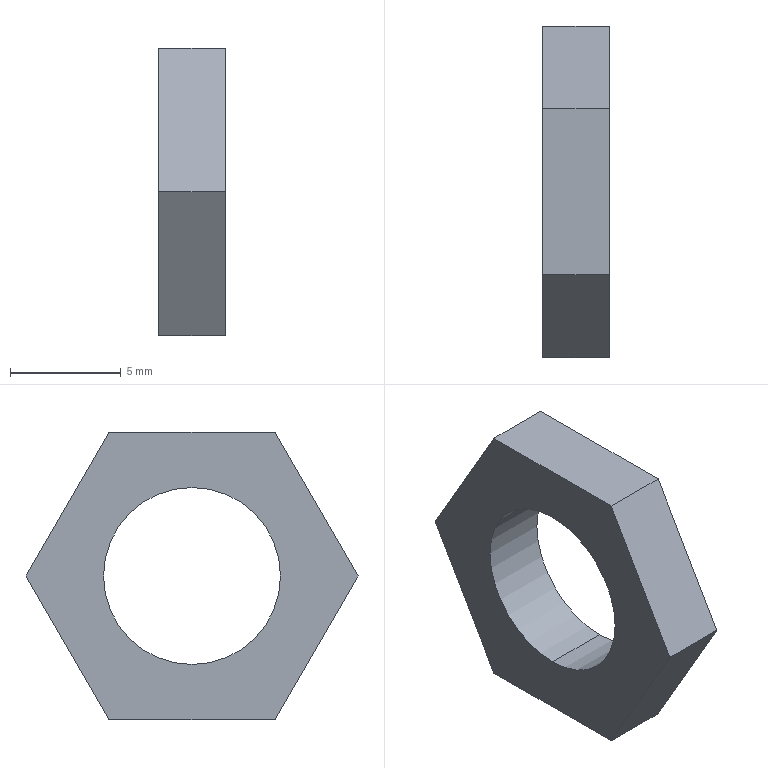Part | STEP file | E2E_X2D1_N_NUT | 1 solid | 10 faces | box 3 x 15.011 x 13 mm | volume 288.278 mm3 | plane 8 | cylinder 2 | commonest cylinder face diameters 8 x2
STEP:
#1=CARTESIAN_POINT('',(0.,0.,0.));
#2=DIRECTION('',(0.,0.,1.));
#3=DIRECTION('',(1.,0.,0.));
#4=AXIS2_PLACEMENT_3D('',#1,#2,#3);
#5=CARTESIAN_POINT('',(3.,0.,4.));
#6=VERTEX_POINT('',#5);
#7=CARTESIAN_POINT('',(0.,0.,4.));
#8=VERTEX_POINT('',#7);
#9=CARTESIAN_POINT('',(3.,0.,4.));
#10=DIRECTION('',(-1.,0.,0.));
#11=VECTOR('',#10,1.);
#12=LINE('',#9,#11);
#13=CARTESIAN_POINT('',(3.,0.,0.));
#14=DIRECTION('',(-1.,0.,0.));
#15=DIRECTION('',(0.,0.,1.));
#16=AXIS2_PLACEMENT_3D('',#13,#14,#15);
#17=CYLINDRICAL_SURFACE('',#16,4.);
#18=CARTESIAN_POINT('',(6.283,0.));
#19=DIRECTION('',(0.,1.));
#20=VECTOR('',#19,1.);
#21=LINE('',#18,#20);
#22=(GEOMETRIC_REPRESENTATION_CONTEXT(2)PARAMETRIC_REPRESENTATION_CONTEXT()REPRESENTATION_CONTEXT('',''));
#23=DEFINITIONAL_REPRESENTATION('',(#21),#22);
#24=PCURVE('',#17,#23);
#25=CARTESIAN_POINT('',(3.,0.,0.));
#26=DIRECTION('',(-1.,0.,0.));
#27=DIRECTION('',(0.,0.,1.));
#28=AXIS2_PLACEMENT_3D('',#25,#26,#27);
#29=CYLINDRICAL_SURFACE('',#28,4.);
#30=CARTESIAN_POINT('',(0.,0.));
#31=DIRECTION('',(0.,1.));
#32=VECTOR('',#31,1.);
#33=LINE('',#30,#32);
#34=(GEOMETRIC_REPRESENTATION_CONTEXT(2)PARAMETRIC_REPRESENTATION_CONTEXT()REPRESENTATION_CONTEXT('',''));
#35=DEFINITIONAL_REPRESENTATION('',(#33),#34);
#36=PCURVE('',#29,#35);
#37=SURFACE_CURVE('',#12,(#24,#36),.PCURVE_S1.);
#38=EDGE_CURVE('',#6,#8,#37,.T.);
#39=ORIENTED_EDGE('',*,*,#38,.T.);
#40=CARTESIAN_POINT('',(0.,0.,-4.));
#41=VERTEX_POINT('',#40);
#42=CARTESIAN_POINT('',(0.,0.,0.));
#43=DIRECTION('',(1.,0.,0.));
#44=DIRECTION('',(0.,0.,-1.));
#45=AXIS2_PLACEMENT_3D('',#42,#43,#44);
#46=CIRCLE('',#45,4.);
#47=CARTESIAN_POINT('',(9.425,3.));
#48=DIRECTION('',(-1.,0.));
#49=VECTOR('',#48,1.);
#50=LINE('',#47,#49);
#51=(GEOMETRIC_REPRESENTATION_CONTEXT(2)PARAMETRIC_REPRESENTATION_CONTEXT()REPRESENTATION_CONTEXT('',''));
#52=DEFINITIONAL_REPRESENTATION('',(#50),#51);
#53=PCURVE('',#17,#52);
#54=CARTESIAN_POINT('',(0.,-3.753,-6.5));
#55=DIRECTION('',(1.,0.,0.));
#56=DIRECTION('',(0.,0.,-1.));
#57=AXIS2_PLACEMENT_3D('',#54,#55,#56);
#58=PLANE('',#57);
#59=CARTESIAN_POINT('',(-6.5,3.753));
#60=DIRECTION('',(1.,0.));
#61=AXIS2_PLACEMENT_2D('',#59,#60);
#62=CIRCLE('',#61,4.);
#63=(GEOMETRIC_REPRESENTATION_CONTEXT(2)PARAMETRIC_REPRESENTATION_CONTEXT()REPRESENTATION_CONTEXT('',''));
#64=DEFINITIONAL_REPRESENTATION('',(#62),#63);
#65=PCURVE('',#58,#64);
#66=SURFACE_CURVE('',#46,(#53,#65),.PCURVE_S1.);
#67=EDGE_CURVE('',#8,#41,#66,.T.);
#68=ORIENTED_EDGE('',*,*,#67,.T.);
#69=CARTESIAN_POINT('',(3.,0.,-4.));
#70=VERTEX_POINT('',#69);
#71=CARTESIAN_POINT('',(3.,0.,-4.));
#72=DIRECTION('',(-1.,0.,0.));
#73=VECTOR('',#72,1.);
#74=LINE('',#71,#73);
#75=CARTESIAN_POINT('',(3.142,0.));
#76=DIRECTION('',(0.,1.));
#77=VECTOR('',#76,1.);
#78=LINE('',#75,#77);
#79=(GEOMETRIC_REPRESENTATION_CONTEXT(2)PARAMETRIC_REPRESENTATION_CONTEXT()REPRESENTATION_CONTEXT('',''));
#80=DEFINITIONAL_REPRESENTATION('',(#78),#79);
#81=PCURVE('',#17,#80);
#82=CARTESIAN_POINT('',(3.142,0.));
#83=DIRECTION('',(0.,1.));
#84=VECTOR('',#83,1.);
#85=LINE('',#82,#84);
#86=(GEOMETRIC_REPRESENTATION_CONTEXT(2)PARAMETRIC_REPRESENTATION_CONTEXT()REPRESENTATION_CONTEXT('',''));
#87=DEFINITIONAL_REPRESENTATION('',(#85),#86);
#88=PCURVE('',#29,#87);
#89=SURFACE_CURVE('',#74,(#81,#88),.PCURVE_S1.);
#90=EDGE_CURVE('',#70,#41,#89,.T.);
#91=ORIENTED_EDGE('',*,*,#90,.F.);
#92=CARTESIAN_POINT('',(3.,0.,0.));
#93=DIRECTION('',(1.,0.,0.));
#94=DIRECTION('',(0.,0.,-1.));
#95=AXIS2_PLACEMENT_3D('',#92,#93,#94);
#96=CIRCLE('',#95,4.);
#97=CARTESIAN_POINT('',(9.425,0.));
#98=DIRECTION('',(-1.,0.));
#99=VECTOR('',#98,1.);
#100=LINE('',#97,#99);
#101=(GEOMETRIC_REPRESENTATION_CONTEXT(2)PARAMETRIC_REPRESENTATION_CONTEXT()REPRESENTATION_CONTEXT('',''));
#102=DEFINITIONAL_REPRESENTATION('',(#100),#101);
#103=PCURVE('',#17,#102);
#104=CARTESIAN_POINT('',(3.,-3.753,-6.5));
#105=DIRECTION('',(1.,0.,0.));
#106=DIRECTION('',(0.,0.,-1.));
#107=AXIS2_PLACEMENT_3D('',#104,#105,#106);
#108=PLANE('',#107);
#109=CARTESIAN_POINT('',(-6.5,3.753));
#110=DIRECTION('',(1.,0.));
#111=AXIS2_PLACEMENT_2D('',#109,#110);
#112=CIRCLE('',#111,4.);
#113=(GEOMETRIC_REPRESENTATION_CONTEXT(2)PARAMETRIC_REPRESENTATION_CONTEXT()REPRESENTATION_CONTEXT('',''));
#114=DEFINITIONAL_REPRESENTATION('',(#112),#113);
#115=PCURVE('',#108,#114);
#116=SURFACE_CURVE('',#96,(#103,#115),.PCURVE_S1.);
#117=EDGE_CURVE('',#6,#70,#116,.T.);
#118=ORIENTED_EDGE('',*,*,#117,.F.);
#119=EDGE_LOOP('',(#39,#68,#91,#118));
#120=FACE_BOUND('',#119,.F.);
#121=ADVANCED_FACE('',(#120),#17,.F.);
#122=CARTESIAN_POINT('',(3.,-7.506,0.));
#123=VERTEX_POINT('',#122);
#124=CARTESIAN_POINT('',(3.,-3.753,-6.5));
#125=VERTEX_POINT('',#124);
#126=CARTESIAN_POINT('',(3.,-7.506,0.));
#127=DIRECTION('',(0.,0.5,-0.866));
#128=VECTOR('',#127,1.);
#129=LINE('',#126,#128);
#130=CARTESIAN_POINT('',(-6.5,-3.753));
#131=DIRECTION('',(0.866,0.5));
#132=VECTOR('',#131,1.);
#133=LINE('',#130,#132);
#134=(GEOMETRIC_REPRESENTATION_CONTEXT(2)PARAMETRIC_REPRESENTATION_CONTEXT()REPRESENTATION_CONTEXT('',''));
#135=DEFINITIONAL_REPRESENTATION('',(#133),#134);
#136=PCURVE('',#108,#135);
#137=CARTESIAN_POINT('',(3.,-7.506,0.));
#138=DIRECTION('',(0.,0.866,0.5));
#139=DIRECTION('',(0.,-0.5,0.866));
#140=AXIS2_PLACEMENT_3D('',#137,#138,#139);
#141=PLANE('',#140);
#142=CARTESIAN_POINT('',(0.,0.));
#143=DIRECTION('',(-1.,0.));
#144=VECTOR('',#143,1.);
#145=LINE('',#142,#144);
#146=(GEOMETRIC_REPRESENTATION_CONTEXT(2)PARAMETRIC_REPRESENTATION_CONTEXT()REPRESENTATION_CONTEXT('',''));
#147=DEFINITIONAL_REPRESENTATION('',(#145),#146);
#148=PCURVE('',#141,#147);
#149=SURFACE_CURVE('',#129,(#136,#148),.PCURVE_S1.);
#150=EDGE_CURVE('',#123,#125,#149,.T.);
#151=ORIENTED_EDGE('',*,*,#150,.T.);
#152=CARTESIAN_POINT('',(3.,3.753,-6.5));
#153=VERTEX_POINT('',#152);
#154=CARTESIAN_POINT('',(3.,-3.753,-6.5));
#155=DIRECTION('',(0.,1.,0.));
#156=VECTOR('',#155,1.);
#157=LINE('',#154,#156);
#158=CARTESIAN_POINT('',(0.,0.));
#159=DIRECTION('',(0.,1.));
#160=VECTOR('',#159,1.);
#161=LINE('',#158,#160);
#162=(GEOMETRIC_REPRESENTATION_CONTEXT(2)PARAMETRIC_REPRESENTATION_CONTEXT()REPRESENTATION_CONTEXT('',''));
#163=DEFINITIONAL_REPRESENTATION('',(#161),#162);
#164=PCURVE('',#108,#163);
#165=CARTESIAN_POINT('',(3.,-3.753,-6.5));
#166=DIRECTION('',(0.,0.,1.));
#167=DIRECTION('',(1.,0.,0.));
#168=AXIS2_PLACEMENT_3D('',#165,#166,#167);
#169=PLANE('',#168);
#170=CARTESIAN_POINT('',(0.,0.));
#171=DIRECTION('',(0.,1.));
#172=VECTOR('',#171,1.);
#173=LINE('',#170,#172);
#174=(GEOMETRIC_REPRESENTATION_CONTEXT(2)PARAMETRIC_REPRESENTATION_CONTEXT()REPRESENTATION_CONTEXT('',''));
#175=DEFINITIONAL_REPRESENTATION('',(#173),#174);
#176=PCURVE('',#169,#175);
#177=SURFACE_CURVE('',#157,(#164,#176),.PCURVE_S1.);
#178=EDGE_CURVE('',#125,#153,#177,.T.);
#179=ORIENTED_EDGE('',*,*,#178,.T.);
#180=CARTESIAN_POINT('',(3.,7.506,0.));
#181=VERTEX_POINT('',#180);
#182=CARTESIAN_POINT('',(3.,3.753,-6.5));
#183=DIRECTION('',(0.,0.5,0.866));
#184=VECTOR('',#183,1.);
#185=LINE('',#182,#184);
#186=CARTESIAN_POINT('',(0.,7.506));
#187=DIRECTION('',(-0.866,0.5));
#188=VECTOR('',#187,1.);
#189=LINE('',#186,#188);
#190=(GEOMETRIC_REPRESENTATION_CONTEXT(2)PARAMETRIC_REPRESENTATION_CONTEXT()REPRESENTATION_CONTEXT('',''));
#191=DEFINITIONAL_REPRESENTATION('',(#189),#190);
#192=PCURVE('',#108,#191);
#193=CARTESIAN_POINT('',(3.,3.753,-6.5));
#194=DIRECTION('',(0.,-0.866,0.5));
#195=DIRECTION('',(0.,-0.5,-0.866));
#196=AXIS2_PLACEMENT_3D('',#193,#194,#195);
#197=PLANE('',#196);
#198=CARTESIAN_POINT('',(0.,0.));
#199=DIRECTION('',(-1.,0.));
#200=VECTOR('',#199,1.);
#201=LINE('',#198,#200);
#202=(GEOMETRIC_REPRESENTATION_CONTEXT(2)PARAMETRIC_REPRESENTATION_CONTEXT()REPRESENTATION_CONTEXT('',''));
#203=DEFINITIONAL_REPRESENTATION('',(#201),#202);
#204=PCURVE('',#197,#203);
#205=SURFACE_CURVE('',#185,(#192,#204),.PCURVE_S1.);
#206=EDGE_CURVE('',#153,#181,#205,.T.);
#207=ORIENTED_EDGE('',*,*,#206,.T.);
#208=CARTESIAN_POINT('',(3.,3.753,6.5));
#209=VERTEX_POINT('',#208);
#210=CARTESIAN_POINT('',(3.,7.506,0.));
#211=DIRECTION('',(0.,-0.5,0.866));
#212=VECTOR('',#211,1.);
#213=LINE('',#210,#212);
#214=CARTESIAN_POINT('',(-6.5,11.258));
#215=DIRECTION('',(-0.866,-0.5));
#216=VECTOR('',#215,1.);
#217=LINE('',#214,#216);
#218=(GEOMETRIC_REPRESENTATION_CONTEXT(2)PARAMETRIC_REPRESENTATION_CONTEXT()REPRESENTATION_CONTEXT('',''));
#219=DEFINITIONAL_REPRESENTATION('',(#217),#218);
#220=PCURVE('',#108,#219);
#221=CARTESIAN_POINT('',(3.,7.506,0.));
#222=DIRECTION('',(0.,-0.866,-0.5));
#223=DIRECTION('',(0.,0.5,-0.866));
#224=AXIS2_PLACEMENT_3D('',#221,#222,#223);
#225=PLANE('',#224);
#226=CARTESIAN_POINT('',(0.,0.));
#227=DIRECTION('',(-1.,0.));
#228=VECTOR('',#227,1.);
#229=LINE('',#226,#228);
#230=(GEOMETRIC_REPRESENTATION_CONTEXT(2)PARAMETRIC_REPRESENTATION_CONTEXT()REPRESENTATION_CONTEXT('',''));
#231=DEFINITIONAL_REPRESENTATION('',(#229),#230);
#232=PCURVE('',#225,#231);
#233=SURFACE_CURVE('',#213,(#220,#232),.PCURVE_S1.);
#234=EDGE_CURVE('',#181,#209,#233,.T.);
#235=ORIENTED_EDGE('',*,*,#234,.T.);
#236=CARTESIAN_POINT('',(3.,-3.753,6.5));
#237=VERTEX_POINT('',#236);
#238=CARTESIAN_POINT('',(3.,3.753,6.5));
#239=DIRECTION('',(0.,-1.,0.));
#240=VECTOR('',#239,1.);
#241=LINE('',#238,#240);
#242=CARTESIAN_POINT('',(-13.,7.506));
#243=DIRECTION('',(0.,-1.));
#244=VECTOR('',#243,1.);
#245=LINE('',#242,#244);
#246=(GEOMETRIC_REPRESENTATION_CONTEXT(2)PARAMETRIC_REPRESENTATION_CONTEXT()REPRESENTATION_CONTEXT('',''));
#247=DEFINITIONAL_REPRESENTATION('',(#245),#246);
#248=PCURVE('',#108,#247);
#249=CARTESIAN_POINT('',(3.,3.753,6.5));
#250=DIRECTION('',(0.,0.,-1.));
#251=DIRECTION('',(0.,1.,0.));
#252=AXIS2_PLACEMENT_3D('',#249,#250,#251);
#253=PLANE('',#252);
#254=CARTESIAN_POINT('',(0.,0.));
#255=DIRECTION('',(-1.,0.));
#256=VECTOR('',#255,1.);
#257=LINE('',#254,#256);
#258=(GEOMETRIC_REPRESENTATION_CONTEXT(2)PARAMETRIC_REPRESENTATION_CONTEXT()REPRESENTATION_CONTEXT('',''));
#259=DEFINITIONAL_REPRESENTATION('',(#257),#258);
#260=PCURVE('',#253,#259);
#261=SURFACE_CURVE('',#241,(#248,#260),.PCURVE_S1.);
#262=EDGE_CURVE('',#209,#237,#261,.T.);
#263=ORIENTED_EDGE('',*,*,#262,.T.);
#264=CARTESIAN_POINT('',(3.,-3.753,6.5));
#265=DIRECTION('',(0.,-0.5,-0.866));
#266=VECTOR('',#265,1.);
#267=LINE('',#264,#266);
#268=CARTESIAN_POINT('',(-13.,0.));
#269=DIRECTION('',(0.866,-0.5));
#270=VECTOR('',#269,1.);
#271=LINE('',#268,#270);
#272=(GEOMETRIC_REPRESENTATION_CONTEXT(2)PARAMETRIC_REPRESENTATION_CONTEXT()REPRESENTATION_CONTEXT('',''));
#273=DEFINITIONAL_REPRESENTATION('',(#271),#272);
#274=PCURVE('',#108,#273);
#275=CARTESIAN_POINT('',(3.,-3.753,6.5));
#276=DIRECTION('',(0.,0.866,-0.5));
#277=DIRECTION('',(0.,0.5,0.866));
#278=AXIS2_PLACEMENT_3D('',#275,#276,#277);
#279=PLANE('',#278);
#280=CARTESIAN_POINT('',(0.,0.));
#281=DIRECTION('',(-1.,0.));
#282=VECTOR('',#281,1.);
#283=LINE('',#280,#282);
#284=(GEOMETRIC_REPRESENTATION_CONTEXT(2)PARAMETRIC_REPRESENTATION_CONTEXT()REPRESENTATION_CONTEXT('',''));
#285=DEFINITIONAL_REPRESENTATION('',(#283),#284);
#286=PCURVE('',#279,#285);
#287=SURFACE_CURVE('',#267,(#274,#286),.PCURVE_S1.);
#288=EDGE_CURVE('',#237,#123,#287,.T.);
#289=ORIENTED_EDGE('',*,*,#288,.T.);
#290=EDGE_LOOP('',(#151,#179,#207,#235,#263,#289));
#291=FACE_BOUND('',#290,.T.);
#292=ORIENTED_EDGE('',*,*,#117,.F.);
#293=CARTESIAN_POINT('',(3.,0.,0.));
#294=DIRECTION('',(1.,0.,0.));
#295=DIRECTION('',(0.,0.,-1.));
#296=AXIS2_PLACEMENT_3D('',#293,#294,#295);
#297=CIRCLE('',#296,4.);
#298=CARTESIAN_POINT('',(-6.5,3.753));
#299=DIRECTION('',(1.,0.));
#300=AXIS2_PLACEMENT_2D('',#298,#299);
#301=CIRCLE('',#300,4.);
#302=(GEOMETRIC_REPRESENTATION_CONTEXT(2)PARAMETRIC_REPRESENTATION_CONTEXT()REPRESENTATION_CONTEXT('',''));
#303=DEFINITIONAL_REPRESENTATION('',(#301),#302);
#304=PCURVE('',#108,#303);
#305=CARTESIAN_POINT('',(3.142,0.));
#306=DIRECTION('',(-1.,0.));
#307=VECTOR('',#306,1.);
#308=LINE('',#305,#307);
#309=(GEOMETRIC_REPRESENTATION_CONTEXT(2)PARAMETRIC_REPRESENTATION_CONTEXT()REPRESENTATION_CONTEXT('',''));
#310=DEFINITIONAL_REPRESENTATION('',(#308),#309);
#311=PCURVE('',#29,#310);
#312=SURFACE_CURVE('',#297,(#304,#311),.PCURVE_S1.);
#313=EDGE_CURVE('',#70,#6,#312,.T.);
#314=ORIENTED_EDGE('',*,*,#313,.F.);
#315=EDGE_LOOP('',(#292,#314));
#316=FACE_BOUND('',#315,.T.);
#317=ADVANCED_FACE('',(#291,#316),#108,.T.);
#318=CARTESIAN_POINT('',(0.,-7.506,0.));
#319=VERTEX_POINT('',#318);
#320=CARTESIAN_POINT('',(0.,-3.753,-6.5));
#321=VERTEX_POINT('',#320);
#322=CARTESIAN_POINT('',(0.,-7.506,0.));
#323=DIRECTION('',(0.,0.5,-0.866));
#324=VECTOR('',#323,1.);
#325=LINE('',#322,#324);
#326=CARTESIAN_POINT('',(-6.5,-3.753));
#327=DIRECTION('',(0.866,0.5));
#328=VECTOR('',#327,1.);
#329=LINE('',#326,#328);
#330=(GEOMETRIC_REPRESENTATION_CONTEXT(2)PARAMETRIC_REPRESENTATION_CONTEXT()REPRESENTATION_CONTEXT('',''));
#331=DEFINITIONAL_REPRESENTATION('',(#329),#330);
#332=PCURVE('',#58,#331);
#333=CARTESIAN_POINT('',(0.,-3.));
#334=DIRECTION('',(-1.,0.));
#335=VECTOR('',#334,1.);
#336=LINE('',#333,#335);
#337=(GEOMETRIC_REPRESENTATION_CONTEXT(2)PARAMETRIC_REPRESENTATION_CONTEXT()REPRESENTATION_CONTEXT('',''));
#338=DEFINITIONAL_REPRESENTATION('',(#336),#337);
#339=PCURVE('',#141,#338);
#340=SURFACE_CURVE('',#325,(#332,#339),.PCURVE_S1.);
#341=EDGE_CURVE('',#319,#321,#340,.T.);
#342=ORIENTED_EDGE('',*,*,#341,.F.);
#343=CARTESIAN_POINT('',(0.,-3.753,6.5));
#344=VERTEX_POINT('',#343);
#345=CARTESIAN_POINT('',(0.,-3.753,6.5));
#346=DIRECTION('',(0.,-0.5,-0.866));
#347=VECTOR('',#346,1.);
#348=LINE('',#345,#347);
#349=CARTESIAN_POINT('',(-13.,0.));
#350=DIRECTION('',(0.866,-0.5));
#351=VECTOR('',#350,1.);
#352=LINE('',#349,#351);
#353=(GEOMETRIC_REPRESENTATION_CONTEXT(2)PARAMETRIC_REPRESENTATION_CONTEXT()REPRESENTATION_CONTEXT('',''));
#354=DEFINITIONAL_REPRESENTATION('',(#352),#353);
#355=PCURVE('',#58,#354);
#356=CARTESIAN_POINT('',(0.,-3.));
#357=DIRECTION('',(-1.,0.));
#358=VECTOR('',#357,1.);
#359=LINE('',#356,#358);
#360=(GEOMETRIC_REPRESENTATION_CONTEXT(2)PARAMETRIC_REPRESENTATION_CONTEXT()REPRESENTATION_CONTEXT('',''));
#361=DEFINITIONAL_REPRESENTATION('',(#359),#360);
#362=PCURVE('',#279,#361);
#363=SURFACE_CURVE('',#348,(#355,#362),.PCURVE_S1.);
#364=EDGE_CURVE('',#344,#319,#363,.T.);
#365=ORIENTED_EDGE('',*,*,#364,.F.);
#366=CARTESIAN_POINT('',(0.,3.753,6.5));
#367=VERTEX_POINT('',#366);
#368=CARTESIAN_POINT('',(0.,3.753,6.5));
#369=DIRECTION('',(0.,-1.,0.));
#370=VECTOR('',#369,1.);
#371=LINE('',#368,#370);
#372=CARTESIAN_POINT('',(-13.,7.506));
#373=DIRECTION('',(0.,-1.));
#374=VECTOR('',#373,1.);
#375=LINE('',#372,#374);
#376=(GEOMETRIC_REPRESENTATION_CONTEXT(2)PARAMETRIC_REPRESENTATION_CONTEXT()REPRESENTATION_CONTEXT('',''));
#377=DEFINITIONAL_REPRESENTATION('',(#375),#376);
#378=PCURVE('',#58,#377);
#379=CARTESIAN_POINT('',(0.,-3.));
#380=DIRECTION('',(-1.,0.));
#381=VECTOR('',#380,1.);
#382=LINE('',#379,#381);
#383=(GEOMETRIC_REPRESENTATION_CONTEXT(2)PARAMETRIC_REPRESENTATION_CONTEXT()REPRESENTATION_CONTEXT('',''));
#384=DEFINITIONAL_REPRESENTATION('',(#382),#383);
#385=PCURVE('',#253,#384);
#386=SURFACE_CURVE('',#371,(#378,#385),.PCURVE_S1.);
#387=EDGE_CURVE('',#367,#344,#386,.T.);
#388=ORIENTED_EDGE('',*,*,#387,.F.);
#389=CARTESIAN_POINT('',(0.,7.506,0.));
#390=VERTEX_POINT('',#389);
#391=CARTESIAN_POINT('',(0.,7.506,0.));
#392=DIRECTION('',(0.,-0.5,0.866));
#393=VECTOR('',#392,1.);
#394=LINE('',#391,#393);
#395=CARTESIAN_POINT('',(-6.5,11.258));
#396=DIRECTION('',(-0.866,-0.5));
#397=VECTOR('',#396,1.);
#398=LINE('',#395,#397);
#399=(GEOMETRIC_REPRESENTATION_CONTEXT(2)PARAMETRIC_REPRESENTATION_CONTEXT()REPRESENTATION_CONTEXT('',''));
#400=DEFINITIONAL_REPRESENTATION('',(#398),#399);
#401=PCURVE('',#58,#400);
#402=CARTESIAN_POINT('',(0.,-3.));
#403=DIRECTION('',(-1.,0.));
#404=VECTOR('',#403,1.);
#405=LINE('',#402,#404);
#406=(GEOMETRIC_REPRESENTATION_CONTEXT(2)PARAMETRIC_REPRESENTATION_CONTEXT()REPRESENTATION_CONTEXT('',''));
#407=DEFINITIONAL_REPRESENTATION('',(#405),#406);
#408=PCURVE('',#225,#407);
#409=SURFACE_CURVE('',#394,(#401,#408),.PCURVE_S1.);
#410=EDGE_CURVE('',#390,#367,#409,.T.);
#411=ORIENTED_EDGE('',*,*,#410,.F.);
#412=CARTESIAN_POINT('',(0.,3.753,-6.5));
#413=VERTEX_POINT('',#412);
#414=CARTESIAN_POINT('',(0.,3.753,-6.5));
#415=DIRECTION('',(0.,0.5,0.866));
#416=VECTOR('',#415,1.);
#417=LINE('',#414,#416);
#418=CARTESIAN_POINT('',(0.,7.506));
#419=DIRECTION('',(-0.866,0.5));
#420=VECTOR('',#419,1.);
#421=LINE('',#418,#420);
#422=(GEOMETRIC_REPRESENTATION_CONTEXT(2)PARAMETRIC_REPRESENTATION_CONTEXT()REPRESENTATION_CONTEXT('',''));
#423=DEFINITIONAL_REPRESENTATION('',(#421),#422);
#424=PCURVE('',#58,#423);
#425=CARTESIAN_POINT('',(0.,-3.));
#426=DIRECTION('',(-1.,0.));
#427=VECTOR('',#426,1.);
#428=LINE('',#425,#427);
#429=(GEOMETRIC_REPRESENTATION_CONTEXT(2)PARAMETRIC_REPRESENTATION_CONTEXT()REPRESENTATION_CONTEXT('',''));
#430=DEFINITIONAL_REPRESENTATION('',(#428),#429);
#431=PCURVE('',#197,#430);
#432=SURFACE_CURVE('',#417,(#424,#431),.PCURVE_S1.);
#433=EDGE_CURVE('',#413,#390,#432,.T.);
#434=ORIENTED_EDGE('',*,*,#433,.F.);
#435=CARTESIAN_POINT('',(0.,-3.753,-6.5));
#436=DIRECTION('',(0.,1.,0.));
#437=VECTOR('',#436,1.);
#438=LINE('',#435,#437);
#439=CARTESIAN_POINT('',(0.,0.));
#440=DIRECTION('',(0.,1.));
#441=VECTOR('',#440,1.);
#442=LINE('',#439,#441);
#443=(GEOMETRIC_REPRESENTATION_CONTEXT(2)PARAMETRIC_REPRESENTATION_CONTEXT()REPRESENTATION_CONTEXT('',''));
#444=DEFINITIONAL_REPRESENTATION('',(#442),#443);
#445=PCURVE('',#58,#444);
#446=CARTESIAN_POINT('',(-3.,0.));
#447=DIRECTION('',(0.,1.));
#448=VECTOR('',#447,1.);
#449=LINE('',#446,#448);
#450=(GEOMETRIC_REPRESENTATION_CONTEXT(2)PARAMETRIC_REPRESENTATION_CONTEXT()REPRESENTATION_CONTEXT('',''));
#451=DEFINITIONAL_REPRESENTATION('',(#449),#450);
#452=PCURVE('',#169,#451);
#453=SURFACE_CURVE('',#438,(#445,#452),.PCURVE_S1.);
#454=EDGE_CURVE('',#321,#413,#453,.T.);
#455=ORIENTED_EDGE('',*,*,#454,.F.);
#456=EDGE_LOOP('',(#342,#365,#388,#411,#434,#455));
#457=FACE_BOUND('',#456,.T.);
#458=ORIENTED_EDGE('',*,*,#67,.T.);
#459=CARTESIAN_POINT('',(0.,0.,0.));
#460=DIRECTION('',(1.,0.,0.));
#461=DIRECTION('',(0.,0.,-1.));
#462=AXIS2_PLACEMENT_3D('',#459,#460,#461);
#463=CIRCLE('',#462,4.);
#464=CARTESIAN_POINT('',(-6.5,3.753));
#465=DIRECTION('',(1.,0.));
#466=AXIS2_PLACEMENT_2D('',#464,#465);
#467=CIRCLE('',#466,4.);
#468=(GEOMETRIC_REPRESENTATION_CONTEXT(2)PARAMETRIC_REPRESENTATION_CONTEXT()REPRESENTATION_CONTEXT('',''));
#469=DEFINITIONAL_REPRESENTATION('',(#467),#468);
#470=PCURVE('',#58,#469);
#471=CARTESIAN_POINT('',(3.142,3.));
#472=DIRECTION('',(-1.,0.));
#473=VECTOR('',#472,1.);
#474=LINE('',#471,#473);
#475=(GEOMETRIC_REPRESENTATION_CONTEXT(2)PARAMETRIC_REPRESENTATION_CONTEXT()REPRESENTATION_CONTEXT('',''));
#476=DEFINITIONAL_REPRESENTATION('',(#474),#475);
#477=PCURVE('',#29,#476);
#478=SURFACE_CURVE('',#463,(#470,#477),.PCURVE_S1.);
#479=EDGE_CURVE('',#41,#8,#478,.T.);
#480=ORIENTED_EDGE('',*,*,#479,.T.);
#481=EDGE_LOOP('',(#458,#480));
#482=FACE_BOUND('',#481,.T.);
#483=ADVANCED_FACE('',(#457,#482),#58,.F.);
#484=ORIENTED_EDGE('',*,*,#341,.T.);
#485=CARTESIAN_POINT('',(3.,-3.753,-6.5));
#486=DIRECTION('',(-1.,0.,0.));
#487=VECTOR('',#486,1.);
#488=LINE('',#485,#487);
#489=CARTESIAN_POINT('',(-7.506,0.));
#490=DIRECTION('',(0.,-1.));
#491=VECTOR('',#490,1.);
#492=LINE('',#489,#491);
#493=(GEOMETRIC_REPRESENTATION_CONTEXT(2)PARAMETRIC_REPRESENTATION_CONTEXT()REPRESENTATION_CONTEXT('',''));
#494=DEFINITIONAL_REPRESENTATION('',(#492),#493);
#495=PCURVE('',#141,#494);
#496=CARTESIAN_POINT('',(0.,0.));
#497=DIRECTION('',(-1.,0.));
#498=VECTOR('',#497,1.);
#499=LINE('',#496,#498);
#500=(GEOMETRIC_REPRESENTATION_CONTEXT(2)PARAMETRIC_REPRESENTATION_CONTEXT()REPRESENTATION_CONTEXT('',''));
#501=DEFINITIONAL_REPRESENTATION('',(#499),#500);
#502=PCURVE('',#169,#501);
#503=SURFACE_CURVE('',#488,(#495,#502),.PCURVE_S1.);
#504=EDGE_CURVE('',#125,#321,#503,.T.);
#505=ORIENTED_EDGE('',*,*,#504,.F.);
#506=ORIENTED_EDGE('',*,*,#150,.F.);
#507=CARTESIAN_POINT('',(3.,-7.506,0.));
#508=DIRECTION('',(-1.,0.,0.));
#509=VECTOR('',#508,1.);
#510=LINE('',#507,#509);
#511=CARTESIAN_POINT('',(0.,0.));
#512=DIRECTION('',(0.,-1.));
#513=VECTOR('',#512,1.);
#514=LINE('',#511,#513);
#515=(GEOMETRIC_REPRESENTATION_CONTEXT(2)PARAMETRIC_REPRESENTATION_CONTEXT()REPRESENTATION_CONTEXT('',''));
#516=DEFINITIONAL_REPRESENTATION('',(#514),#515);
#517=PCURVE('',#141,#516);
#518=CARTESIAN_POINT('',(-7.506,0.));
#519=DIRECTION('',(0.,-1.));
#520=VECTOR('',#519,1.);
#521=LINE('',#518,#520);
#522=(GEOMETRIC_REPRESENTATION_CONTEXT(2)PARAMETRIC_REPRESENTATION_CONTEXT()REPRESENTATION_CONTEXT('',''));
#523=DEFINITIONAL_REPRESENTATION('',(#521),#522);
#524=PCURVE('',#279,#523);
#525=SURFACE_CURVE('',#510,(#517,#524),.PCURVE_S1.);
#526=EDGE_CURVE('',#123,#319,#525,.T.);
#527=ORIENTED_EDGE('',*,*,#526,.T.);
#528=EDGE_LOOP('',(#484,#505,#506,#527));
#529=FACE_BOUND('',#528,.T.);
#530=ADVANCED_FACE('',(#529),#141,.F.);
#531=ORIENTED_EDGE('',*,*,#454,.T.);
#532=CARTESIAN_POINT('',(3.,3.753,-6.5));
#533=DIRECTION('',(-1.,0.,0.));
#534=VECTOR('',#533,1.);
#535=LINE('',#532,#534);
#536=CARTESIAN_POINT('',(0.,7.506));
#537=DIRECTION('',(-1.,0.));
#538=VECTOR('',#537,1.);
#539=LINE('',#536,#538);
#540=(GEOMETRIC_REPRESENTATION_CONTEXT(2)PARAMETRIC_REPRESENTATION_CONTEXT()REPRESENTATION_CONTEXT('',''));
#541=DEFINITIONAL_REPRESENTATION('',(#539),#540);
#542=PCURVE('',#169,#541);
#543=CARTESIAN_POINT('',(0.,0.));
#544=DIRECTION('',(0.,-1.));
#545=VECTOR('',#544,1.);
#546=LINE('',#543,#545);
#547=(GEOMETRIC_REPRESENTATION_CONTEXT(2)PARAMETRIC_REPRESENTATION_CONTEXT()REPRESENTATION_CONTEXT('',''));
#548=DEFINITIONAL_REPRESENTATION('',(#546),#547);
#549=PCURVE('',#197,#548);
#550=SURFACE_CURVE('',#535,(#542,#549),.PCURVE_S1.);
#551=EDGE_CURVE('',#153,#413,#550,.T.);
#552=ORIENTED_EDGE('',*,*,#551,.F.);
#553=ORIENTED_EDGE('',*,*,#178,.F.);
#554=ORIENTED_EDGE('',*,*,#504,.T.);
#555=EDGE_LOOP('',(#531,#552,#553,#554));
#556=FACE_BOUND('',#555,.T.);
#557=ADVANCED_FACE('',(#556),#169,.F.);
#558=ORIENTED_EDGE('',*,*,#433,.T.);
#559=CARTESIAN_POINT('',(3.,7.506,0.));
#560=DIRECTION('',(-1.,0.,0.));
#561=VECTOR('',#560,1.);
#562=LINE('',#559,#561);
#563=CARTESIAN_POINT('',(-7.506,0.));
#564=DIRECTION('',(0.,-1.));
#565=VECTOR('',#564,1.);
#566=LINE('',#563,#565);
#567=(GEOMETRIC_REPRESENTATION_CONTEXT(2)PARAMETRIC_REPRESENTATION_CONTEXT()REPRESENTATION_CONTEXT('',''));
#568=DEFINITIONAL_REPRESENTATION('',(#566),#567);
#569=PCURVE('',#197,#568);
#570=CARTESIAN_POINT('',(0.,0.));
#571=DIRECTION('',(0.,-1.));
#572=VECTOR('',#571,1.);
#573=LINE('',#570,#572);
#574=(GEOMETRIC_REPRESENTATION_CONTEXT(2)PARAMETRIC_REPRESENTATION_CONTEXT()REPRESENTATION_CONTEXT('',''));
#575=DEFINITIONAL_REPRESENTATION('',(#573),#574);
#576=PCURVE('',#225,#575);
#577=SURFACE_CURVE('',#562,(#569,#576),.PCURVE_S1.);
#578=EDGE_CURVE('',#181,#390,#577,.T.);
#579=ORIENTED_EDGE('',*,*,#578,.F.);
#580=ORIENTED_EDGE('',*,*,#206,.F.);
#581=ORIENTED_EDGE('',*,*,#551,.T.);
#582=EDGE_LOOP('',(#558,#579,#580,#581));
#583=FACE_BOUND('',#582,.T.);
#584=ADVANCED_FACE('',(#583),#197,.F.);
#585=ORIENTED_EDGE('',*,*,#410,.T.);
#586=CARTESIAN_POINT('',(3.,3.753,6.5));
#587=DIRECTION('',(-1.,0.,0.));
#588=VECTOR('',#587,1.);
#589=LINE('',#586,#588);
#590=CARTESIAN_POINT('',(-7.506,0.));
#591=DIRECTION('',(0.,-1.));
#592=VECTOR('',#591,1.);
#593=LINE('',#590,#592);
#594=(GEOMETRIC_REPRESENTATION_CONTEXT(2)PARAMETRIC_REPRESENTATION_CONTEXT()REPRESENTATION_CONTEXT('',''));
#595=DEFINITIONAL_REPRESENTATION('',(#593),#594);
#596=PCURVE('',#225,#595);
#597=CARTESIAN_POINT('',(0.,0.));
#598=DIRECTION('',(0.,-1.));
#599=VECTOR('',#598,1.);
#600=LINE('',#597,#599);
#601=(GEOMETRIC_REPRESENTATION_CONTEXT(2)PARAMETRIC_REPRESENTATION_CONTEXT()REPRESENTATION_CONTEXT('',''));
#602=DEFINITIONAL_REPRESENTATION('',(#600),#601);
#603=PCURVE('',#253,#602);
#604=SURFACE_CURVE('',#589,(#596,#603),.PCURVE_S1.);
#605=EDGE_CURVE('',#209,#367,#604,.T.);
#606=ORIENTED_EDGE('',*,*,#605,.F.);
#607=ORIENTED_EDGE('',*,*,#234,.F.);
#608=ORIENTED_EDGE('',*,*,#578,.T.);
#609=EDGE_LOOP('',(#585,#606,#607,#608));
#610=FACE_BOUND('',#609,.T.);
#611=ADVANCED_FACE('',(#610),#225,.F.);
#612=ORIENTED_EDGE('',*,*,#387,.T.);
#613=CARTESIAN_POINT('',(3.,-3.753,6.5));
#614=DIRECTION('',(-1.,0.,0.));
#615=VECTOR('',#614,1.);
#616=LINE('',#613,#615);
#617=CARTESIAN_POINT('',(-7.506,0.));
#618=DIRECTION('',(0.,-1.));
#619=VECTOR('',#618,1.);
#620=LINE('',#617,#619);
#621=(GEOMETRIC_REPRESENTATION_CONTEXT(2)PARAMETRIC_REPRESENTATION_CONTEXT()REPRESENTATION_CONTEXT('',''));
#622=DEFINITIONAL_REPRESENTATION('',(#620),#621);
#623=PCURVE('',#253,#622);
#624=CARTESIAN_POINT('',(0.,0.));
#625=DIRECTION('',(0.,-1.));
#626=VECTOR('',#625,1.);
#627=LINE('',#624,#626);
#628=(GEOMETRIC_REPRESENTATION_CONTEXT(2)PARAMETRIC_REPRESENTATION_CONTEXT()REPRESENTATION_CONTEXT('',''));
#629=DEFINITIONAL_REPRESENTATION('',(#627),#628);
#630=PCURVE('',#279,#629);
#631=SURFACE_CURVE('',#616,(#623,#630),.PCURVE_S1.);
#632=EDGE_CURVE('',#237,#344,#631,.T.);
#633=ORIENTED_EDGE('',*,*,#632,.F.);
#634=ORIENTED_EDGE('',*,*,#262,.F.);
#635=ORIENTED_EDGE('',*,*,#605,.T.);
#636=EDGE_LOOP('',(#612,#633,#634,#635));
#637=FACE_BOUND('',#636,.T.);
#638=ADVANCED_FACE('',(#637),#253,.F.);
#639=ORIENTED_EDGE('',*,*,#364,.T.);
#640=ORIENTED_EDGE('',*,*,#526,.F.);
#641=ORIENTED_EDGE('',*,*,#288,.F.);
#642=ORIENTED_EDGE('',*,*,#632,.T.);
#643=EDGE_LOOP('',(#639,#640,#641,#642));
#644=FACE_BOUND('',#643,.T.);
#645=ADVANCED_FACE('',(#644),#279,.F.);
#646=ORIENTED_EDGE('',*,*,#479,.T.);
#647=ORIENTED_EDGE('',*,*,#38,.F.);
#648=ORIENTED_EDGE('',*,*,#313,.F.);
#649=ORIENTED_EDGE('',*,*,#90,.T.);
#650=EDGE_LOOP('',(#646,#647,#648,#649));
#651=FACE_BOUND('',#650,.F.);
#652=ADVANCED_FACE('',(#651),#29,.F.);
#653=CLOSED_SHELL('',(#121,#317,#483,#530,#557,#584,#611,#638,#645,#652));
#654=MANIFOLD_SOLID_BREP('',#653);
#655=(LENGTH_UNIT()NAMED_UNIT(*)SI_UNIT(.MILLI.,.METRE.));
#656=UNCERTAINTY_MEASURE_WITH_UNIT(LENGTH_MEASURE(0.0000001),#655,'','');
#657=(NAMED_UNIT(*)PLANE_ANGLE_UNIT()SI_UNIT($,.RADIAN.));
#658=(NAMED_UNIT(*)SI_UNIT($,.STERADIAN.)SOLID_ANGLE_UNIT());
#659=(GEOMETRIC_REPRESENTATION_CONTEXT(3)GLOBAL_UNCERTAINTY_ASSIGNED_CONTEXT((#656))GLOBAL_UNIT_ASSIGNED_CONTEXT((#655,#657,#658))REPRESENTATION_CONTEXT('',''));
#660=ADVANCED_BREP_SHAPE_REPRESENTATION('',(#4,#654),#659);